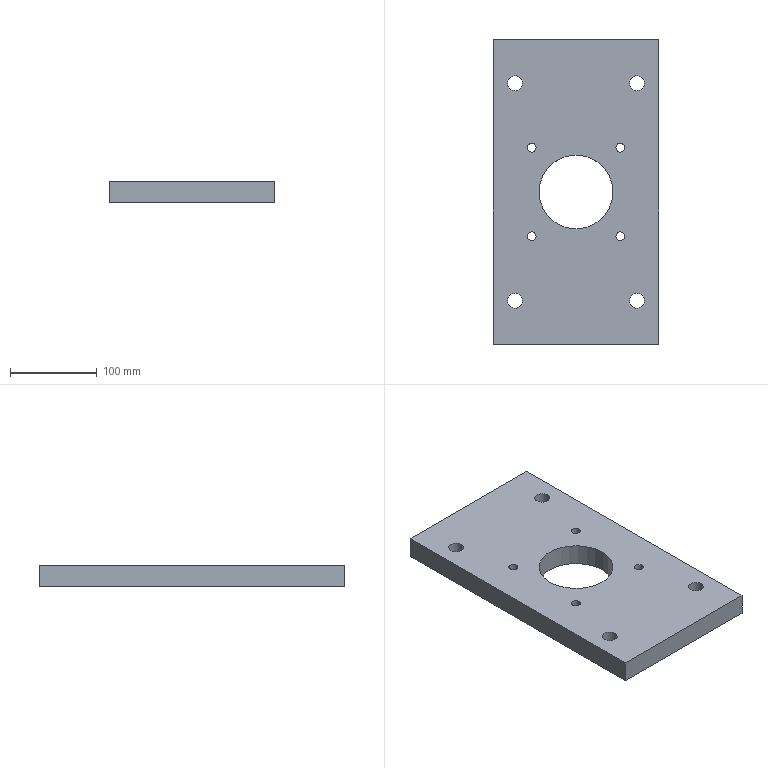Part | STEP file | Bearing housing mounting plate XG | 1 solid | 24 faces | box 190 x 350 x 25 mm | volume 1489768 mm3 | cylinder 18 | plane 6 | commonest cylinder face diameters 10.2 x8 17 x8 85 x2